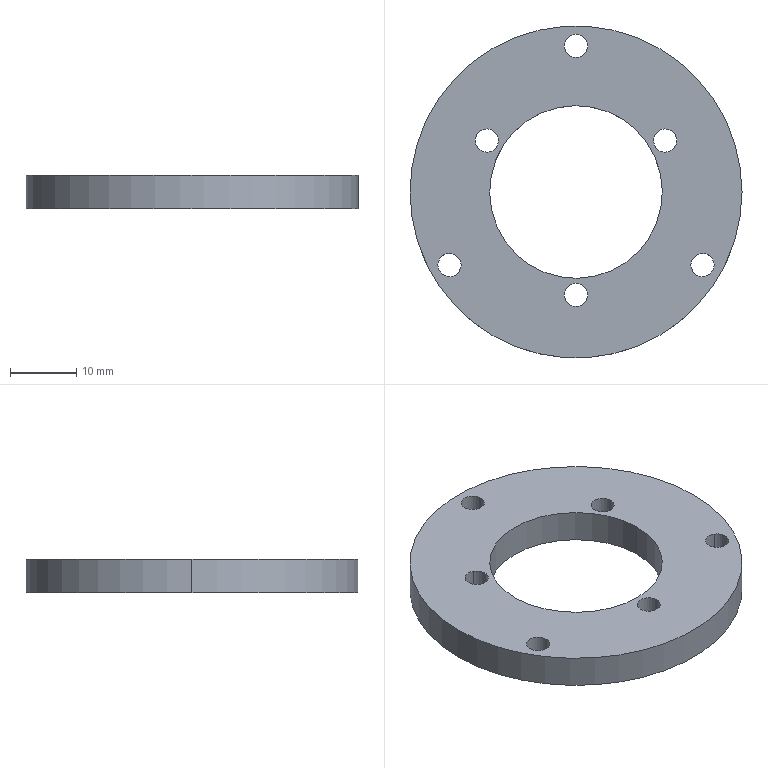Part | SolidWorks | features BaseBody 1 | 1 solid | 18 faces | box 50 x 50 x 5 mm | volume 6874 mm3 | cylinder 16 | plane 2 | commonest cylinder face diameters 3.5 x12 26 x2 50 x2
STEP:
#1=CARTESIAN_POINT('',(326.285,275.622,146.922));
#2=VERTEX_POINT('',#1);
#3=CARTESIAN_POINT('',(328.035,278.653,146.922));
#4=VERTEX_POINT('',#3);
#5=CARTESIAN_POINT('',(327.16,277.138,146.922));
#6=DIRECTION('',(0.,0.,-1.));
#7=DIRECTION('',(0.5,0.866,0.));
#8=AXIS2_PLACEMENT_3D('',#5,#6,#7);
#9=CIRCLE('',#8,1.75);
#10=EDGE_CURVE('',#2,#4,#9,.T.);
#11=ORIENTED_EDGE('',*,*,#10,.F.);
#12=CARTESIAN_POINT('',(326.285,275.622,141.922));
#13=VERTEX_POINT('',#12);
#14=CARTESIAN_POINT('',(326.285,275.622,146.922));
#15=DIRECTION('',(0.,0.,-1.));
#16=VECTOR('',#15,1000.);
#17=LINE('',#14,#16);
#18=EDGE_CURVE('',#2,#13,#17,.T.);
#19=ORIENTED_EDGE('',*,*,#18,.T.);
#20=CARTESIAN_POINT('',(328.035,278.653,141.922));
#21=VERTEX_POINT('',#20);
#22=CARTESIAN_POINT('',(327.16,277.138,141.922));
#23=DIRECTION('',(0.,0.,1.));
#24=DIRECTION('',(-0.5,-0.866,0.));
#25=AXIS2_PLACEMENT_3D('',#22,#23,#24);
#26=CIRCLE('',#25,1.75);
#27=EDGE_CURVE('',#21,#13,#26,.T.);
#28=ORIENTED_EDGE('',*,*,#27,.F.);
#29=CARTESIAN_POINT('',(328.035,278.653,146.922));
#30=DIRECTION('',(0.,0.,-1.));
#31=VECTOR('',#30,1000.);
#32=LINE('',#29,#31);
#33=EDGE_CURVE('',#4,#21,#32,.T.);
#34=ORIENTED_EDGE('',*,*,#33,.F.);
#35=EDGE_LOOP('',(#11,#19,#28,#34));
#36=FACE_OUTER_BOUND('',#35,.T.);
#37=CARTESIAN_POINT('',(327.16,277.138,146.922));
#38=DIRECTION('',(0.,0.,-1.));
#39=DIRECTION('',(0.5,0.866,0.));
#40=AXIS2_PLACEMENT_3D('',#37,#38,#39);
#41=CYLINDRICAL_SURFACE('',#40,1.75);
#42=ADVANCED_FACE('',(#36),#41,.F.);
#43=CARTESIAN_POINT('',(353.132,278.653,146.922));
#44=VERTEX_POINT('',#43);
#45=CARTESIAN_POINT('',(354.882,275.622,146.922));
#46=VERTEX_POINT('',#45);
#47=CARTESIAN_POINT('',(354.007,277.138,146.922));
#48=DIRECTION('',(0.,0.,-1.));
#49=DIRECTION('',(-0.5,0.866,0.));
#50=AXIS2_PLACEMENT_3D('',#47,#48,#49);
#51=CIRCLE('',#50,1.75);
#52=EDGE_CURVE('',#44,#46,#51,.T.);
#53=ORIENTED_EDGE('',*,*,#52,.F.);
#54=CARTESIAN_POINT('',(353.132,278.653,141.922));
#55=VERTEX_POINT('',#54);
#56=CARTESIAN_POINT('',(353.132,278.653,146.922));
#57=DIRECTION('',(0.,0.,-1.));
#58=VECTOR('',#57,1000.);
#59=LINE('',#56,#58);
#60=EDGE_CURVE('',#44,#55,#59,.T.);
#61=ORIENTED_EDGE('',*,*,#60,.T.);
#62=CARTESIAN_POINT('',(354.882,275.622,141.922));
#63=VERTEX_POINT('',#62);
#64=CARTESIAN_POINT('',(354.007,277.138,141.922));
#65=DIRECTION('',(0.,0.,1.));
#66=DIRECTION('',(-0.5,0.866,0.));
#67=AXIS2_PLACEMENT_3D('',#64,#65,#66);
#68=CIRCLE('',#67,1.75);
#69=EDGE_CURVE('',#63,#55,#68,.T.);
#70=ORIENTED_EDGE('',*,*,#69,.F.);
#71=CARTESIAN_POINT('',(354.882,275.622,146.922));
#72=DIRECTION('',(0.,0.,-1.));
#73=VECTOR('',#72,1000.);
#74=LINE('',#71,#73);
#75=EDGE_CURVE('',#46,#63,#74,.T.);
#76=ORIENTED_EDGE('',*,*,#75,.F.);
#77=EDGE_LOOP('',(#53,#61,#70,#76));
#78=FACE_OUTER_BOUND('',#77,.T.);
#79=CARTESIAN_POINT('',(354.007,277.138,146.922));
#80=DIRECTION('',(0.,0.,-1.));
#81=DIRECTION('',(0.5,-0.866,0.));
#82=AXIS2_PLACEMENT_3D('',#79,#80,#81);
#83=CYLINDRICAL_SURFACE('',#82,1.75);
#84=ADVANCED_FACE('',(#78),#83,.F.);
#85=CARTESIAN_POINT('',(342.333,253.888,146.922));
#86=VERTEX_POINT('',#85);
#87=CARTESIAN_POINT('',(338.833,253.888,146.922));
#88=VERTEX_POINT('',#87);
#89=CARTESIAN_POINT('',(340.583,253.888,146.922));
#90=DIRECTION('',(0.,0.,-1.));
#91=DIRECTION('',(1.,0.,0.));
#92=AXIS2_PLACEMENT_3D('',#89,#90,#91);
#93=CIRCLE('',#92,1.75);
#94=EDGE_CURVE('',#86,#88,#93,.T.);
#95=ORIENTED_EDGE('',*,*,#94,.F.);
#96=CARTESIAN_POINT('',(342.333,253.888,141.922));
#97=VERTEX_POINT('',#96);
#98=CARTESIAN_POINT('',(342.333,253.888,146.922));
#99=DIRECTION('',(0.,0.,-1.));
#100=VECTOR('',#99,1000.);
#101=LINE('',#98,#100);
#102=EDGE_CURVE('',#86,#97,#101,.T.);
#103=ORIENTED_EDGE('',*,*,#102,.T.);
#104=CARTESIAN_POINT('',(338.833,253.888,141.922));
#105=VERTEX_POINT('',#104);
#106=CARTESIAN_POINT('',(340.583,253.888,141.922));
#107=DIRECTION('',(0.,0.,1.));
#108=DIRECTION('',(1.,0.,0.));
#109=AXIS2_PLACEMENT_3D('',#106,#107,#108);
#110=CIRCLE('',#109,1.75);
#111=EDGE_CURVE('',#105,#97,#110,.T.);
#112=ORIENTED_EDGE('',*,*,#111,.F.);
#113=CARTESIAN_POINT('',(338.833,253.888,146.922));
#114=DIRECTION('',(0.,0.,-1.));
#115=VECTOR('',#114,1000.);
#116=LINE('',#113,#115);
#117=EDGE_CURVE('',#88,#105,#116,.T.);
#118=ORIENTED_EDGE('',*,*,#117,.F.);
#119=EDGE_LOOP('',(#95,#103,#112,#118));
#120=FACE_OUTER_BOUND('',#119,.T.);
#121=CARTESIAN_POINT('',(340.583,253.888,146.922));
#122=DIRECTION('',(0.,0.,-1.));
#123=DIRECTION('',(-1.,0.,0.));
#124=AXIS2_PLACEMENT_3D('',#121,#122,#123);
#125=CYLINDRICAL_SURFACE('',#124,1.75);
#126=ADVANCED_FACE('',(#120),#125,.F.);
#127=CARTESIAN_POINT('',(358.761,256.872,146.922));
#128=VERTEX_POINT('',#127);
#129=CARTESIAN_POINT('',(360.511,259.903,146.922));
#130=VERTEX_POINT('',#129);
#131=CARTESIAN_POINT('',(359.636,258.388,146.922));
#132=DIRECTION('',(0.,0.,-1.));
#133=DIRECTION('',(-0.5,-0.866,0.));
#134=AXIS2_PLACEMENT_3D('',#131,#132,#133);
#135=CIRCLE('',#134,1.75);
#136=EDGE_CURVE('',#128,#130,#135,.T.);
#137=ORIENTED_EDGE('',*,*,#136,.F.);
#138=CARTESIAN_POINT('',(358.761,256.872,141.922));
#139=VERTEX_POINT('',#138);
#140=CARTESIAN_POINT('',(358.761,256.872,146.922));
#141=DIRECTION('',(0.,0.,-1.));
#142=VECTOR('',#141,1000.);
#143=LINE('',#140,#142);
#144=EDGE_CURVE('',#128,#139,#143,.T.);
#145=ORIENTED_EDGE('',*,*,#144,.T.);
#146=CARTESIAN_POINT('',(360.511,259.903,141.922));
#147=VERTEX_POINT('',#146);
#148=CARTESIAN_POINT('',(359.636,258.388,141.922));
#149=DIRECTION('',(0.,0.,1.));
#150=DIRECTION('',(-0.5,-0.866,0.));
#151=AXIS2_PLACEMENT_3D('',#148,#149,#150);
#152=CIRCLE('',#151,1.75);
#153=EDGE_CURVE('',#147,#139,#152,.T.);
#154=ORIENTED_EDGE('',*,*,#153,.F.);
#155=CARTESIAN_POINT('',(360.511,259.903,146.922));
#156=DIRECTION('',(0.,0.,-1.));
#157=VECTOR('',#156,1000.);
#158=LINE('',#155,#157);
#159=EDGE_CURVE('',#130,#147,#158,.T.);
#160=ORIENTED_EDGE('',*,*,#159,.F.);
#161=EDGE_LOOP('',(#137,#145,#154,#160));
#162=FACE_OUTER_BOUND('',#161,.T.);
#163=CARTESIAN_POINT('',(359.636,258.388,146.922));
#164=DIRECTION('',(0.,0.,-1.));
#165=DIRECTION('',(0.5,0.866,0.));
#166=AXIS2_PLACEMENT_3D('',#163,#164,#165);
#167=CYLINDRICAL_SURFACE('',#166,1.75);
#168=ADVANCED_FACE('',(#162),#167,.F.);
#169=CARTESIAN_POINT('',(320.656,259.903,146.922));
#170=VERTEX_POINT('',#169);
#171=CARTESIAN_POINT('',(322.406,256.872,146.922));
#172=VERTEX_POINT('',#171);
#173=CARTESIAN_POINT('',(321.531,258.388,146.922));
#174=DIRECTION('',(0.,0.,-1.));
#175=DIRECTION('',(-0.5,0.866,0.));
#176=AXIS2_PLACEMENT_3D('',#173,#174,#175);
#177=CIRCLE('',#176,1.75);
#178=EDGE_CURVE('',#170,#172,#177,.T.);
#179=ORIENTED_EDGE('',*,*,#178,.F.);
#180=CARTESIAN_POINT('',(320.656,259.903,141.922));
#181=VERTEX_POINT('',#180);
#182=CARTESIAN_POINT('',(320.656,259.903,146.922));
#183=DIRECTION('',(0.,0.,-1.));
#184=VECTOR('',#183,1000.);
#185=LINE('',#182,#184);
#186=EDGE_CURVE('',#170,#181,#185,.T.);
#187=ORIENTED_EDGE('',*,*,#186,.T.);
#188=CARTESIAN_POINT('',(322.406,256.872,141.922));
#189=VERTEX_POINT('',#188);
#190=CARTESIAN_POINT('',(321.531,258.388,141.922));
#191=DIRECTION('',(0.,0.,1.));
#192=DIRECTION('',(-0.5,0.866,0.));
#193=AXIS2_PLACEMENT_3D('',#190,#191,#192);
#194=CIRCLE('',#193,1.75);
#195=EDGE_CURVE('',#189,#181,#194,.T.);
#196=ORIENTED_EDGE('',*,*,#195,.F.);
#197=CARTESIAN_POINT('',(322.406,256.872,146.922));
#198=DIRECTION('',(0.,0.,-1.));
#199=VECTOR('',#198,1000.);
#200=LINE('',#197,#199);
#201=EDGE_CURVE('',#172,#189,#200,.T.);
#202=ORIENTED_EDGE('',*,*,#201,.F.);
#203=EDGE_LOOP('',(#179,#187,#196,#202));
#204=FACE_OUTER_BOUND('',#203,.T.);
#205=CARTESIAN_POINT('',(321.531,258.388,146.922));
#206=DIRECTION('',(0.,0.,-1.));
#207=DIRECTION('',(0.5,-0.866,0.));
#208=AXIS2_PLACEMENT_3D('',#205,#206,#207);
#209=CYLINDRICAL_SURFACE('',#208,1.75);
#210=ADVANCED_FACE('',(#204),#209,.F.);
#211=CARTESIAN_POINT('',(342.333,291.388,146.922));
#212=VERTEX_POINT('',#211);
#213=CARTESIAN_POINT('',(338.833,291.388,146.922));
#214=VERTEX_POINT('',#213);
#215=CARTESIAN_POINT('',(340.583,291.388,146.922));
#216=DIRECTION('',(0.,0.,-1.));
#217=DIRECTION('',(1.,0.,0.));
#218=AXIS2_PLACEMENT_3D('',#215,#216,#217);
#219=CIRCLE('',#218,1.75);
#220=EDGE_CURVE('',#212,#214,#219,.T.);
#221=ORIENTED_EDGE('',*,*,#220,.F.);
#222=CARTESIAN_POINT('',(342.333,291.388,141.922));
#223=VERTEX_POINT('',#222);
#224=CARTESIAN_POINT('',(342.333,291.388,146.922));
#225=DIRECTION('',(0.,0.,-1.));
#226=VECTOR('',#225,1000.);
#227=LINE('',#224,#226);
#228=EDGE_CURVE('',#212,#223,#227,.T.);
#229=ORIENTED_EDGE('',*,*,#228,.T.);
#230=CARTESIAN_POINT('',(338.833,291.388,141.922));
#231=VERTEX_POINT('',#230);
#232=CARTESIAN_POINT('',(340.583,291.388,141.922));
#233=DIRECTION('',(0.,0.,1.));
#234=DIRECTION('',(1.,0.,0.));
#235=AXIS2_PLACEMENT_3D('',#232,#233,#234);
#236=CIRCLE('',#235,1.75);
#237=EDGE_CURVE('',#231,#223,#236,.T.);
#238=ORIENTED_EDGE('',*,*,#237,.F.);
#239=CARTESIAN_POINT('',(338.833,291.388,146.922));
#240=DIRECTION('',(0.,0.,-1.));
#241=VECTOR('',#240,1000.);
#242=LINE('',#239,#241);
#243=EDGE_CURVE('',#214,#231,#242,.T.);
#244=ORIENTED_EDGE('',*,*,#243,.F.);
#245=EDGE_LOOP('',(#221,#229,#238,#244));
#246=FACE_OUTER_BOUND('',#245,.T.);
#247=CARTESIAN_POINT('',(340.583,291.388,146.922));
#248=DIRECTION('',(0.,0.,-1.));
#249=DIRECTION('',(-1.,0.,0.));
#250=AXIS2_PLACEMENT_3D('',#247,#248,#249);
#251=CYLINDRICAL_SURFACE('',#250,1.75);
#252=ADVANCED_FACE('',(#246),#251,.F.);
#253=CARTESIAN_POINT('',(327.584,269.222,141.922));
#254=VERTEX_POINT('',#253);
#255=CARTESIAN_POINT('',(353.582,269.554,141.922));
#256=VERTEX_POINT('',#255);
#257=CARTESIAN_POINT('',(340.583,269.388,141.922));
#258=DIRECTION('',(0.,0.,1.));
#259=DIRECTION('',(-0.9999,-0.01276,0.));
#260=AXIS2_PLACEMENT_3D('',#257,#258,#259);
#261=CIRCLE('',#260,13.);
#262=EDGE_CURVE('',#254,#256,#261,.T.);
#263=ORIENTED_EDGE('',*,*,#262,.F.);
#264=CARTESIAN_POINT('',(327.584,269.222,146.922));
#265=VERTEX_POINT('',#264);
#266=CARTESIAN_POINT('',(327.584,269.222,68.447));
#267=DIRECTION('',(0.,0.,1.));
#268=VECTOR('',#267,1000.);
#269=LINE('',#266,#268);
#270=EDGE_CURVE('',#254,#265,#269,.T.);
#271=ORIENTED_EDGE('',*,*,#270,.T.);
#272=CARTESIAN_POINT('',(353.582,269.554,146.922));
#273=VERTEX_POINT('',#272);
#274=CARTESIAN_POINT('',(340.583,269.388,146.922));
#275=DIRECTION('',(0.,0.,1.));
#276=DIRECTION('',(-1.,0.,0.));
#277=AXIS2_PLACEMENT_3D('',#274,#275,#276);
#278=CIRCLE('',#277,13.);
#279=EDGE_CURVE('',#265,#273,#278,.T.);
#280=ORIENTED_EDGE('',*,*,#279,.T.);
#281=CARTESIAN_POINT('',(353.582,269.554,68.447));
#282=DIRECTION('',(0.,0.,1.));
#283=VECTOR('',#282,1000.);
#284=LINE('',#281,#283);
#285=EDGE_CURVE('',#256,#273,#284,.T.);
#286=ORIENTED_EDGE('',*,*,#285,.F.);
#287=EDGE_LOOP('',(#263,#271,#280,#286));
#288=FACE_OUTER_BOUND('',#287,.T.);
#289=CARTESIAN_POINT('',(340.583,269.388,68.447));
#290=DIRECTION('',(0.,0.,1.));
#291=DIRECTION('',(0.9999,0.01276,0.));
#292=AXIS2_PLACEMENT_3D('',#289,#290,#291);
#293=CYLINDRICAL_SURFACE('',#292,13.);
#294=ADVANCED_FACE('',(#288),#293,.F.);
#295=CARTESIAN_POINT('',(315.583,269.388,141.922));
#296=VERTEX_POINT('',#295);
#297=CARTESIAN_POINT('',(365.583,269.388,141.922));
#298=VERTEX_POINT('',#297);
#299=CARTESIAN_POINT('',(340.583,269.388,141.922));
#300=DIRECTION('',(0.,0.,-1.));
#301=DIRECTION('',(1.,0.,0.));
#302=AXIS2_PLACEMENT_3D('',#299,#300,#301);
#303=CIRCLE('',#302,25.);
#304=EDGE_CURVE('',#296,#298,#303,.T.);
#305=ORIENTED_EDGE('',*,*,#304,.F.);
#306=CARTESIAN_POINT('',(315.583,269.388,146.922));
#307=VERTEX_POINT('',#306);
#308=CARTESIAN_POINT('',(315.583,269.388,141.922));
#309=DIRECTION('',(0.,0.,1.));
#310=VECTOR('',#309,1000.);
#311=LINE('',#308,#310);
#312=EDGE_CURVE('',#296,#307,#311,.T.);
#313=ORIENTED_EDGE('',*,*,#312,.T.);
#314=CARTESIAN_POINT('',(365.583,269.388,146.922));
#315=VERTEX_POINT('',#314);
#316=CARTESIAN_POINT('',(340.583,269.388,146.922));
#317=DIRECTION('',(0.,0.,1.));
#318=DIRECTION('',(-1.,0.,0.));
#319=AXIS2_PLACEMENT_3D('',#316,#317,#318);
#320=CIRCLE('',#319,25.);
#321=EDGE_CURVE('',#315,#307,#320,.T.);
#322=ORIENTED_EDGE('',*,*,#321,.F.);
#323=CARTESIAN_POINT('',(365.583,269.388,141.922));
#324=DIRECTION('',(0.,0.,1.));
#325=VECTOR('',#324,1000.);
#326=LINE('',#323,#325);
#327=EDGE_CURVE('',#298,#315,#326,.T.);
#328=ORIENTED_EDGE('',*,*,#327,.F.);
#329=EDGE_LOOP('',(#305,#313,#322,#328));
#330=FACE_OUTER_BOUND('',#329,.T.);
#331=CARTESIAN_POINT('',(340.583,269.388,141.922));
#332=DIRECTION('',(0.,0.,1.));
#333=DIRECTION('',(1.,0.,0.));
#334=AXIS2_PLACEMENT_3D('',#331,#332,#333);
#335=CYLINDRICAL_SURFACE('',#334,25.);
#336=ADVANCED_FACE('',(#330),#335,.T.);
#337=ORIENTED_EDGE('',*,*,#312,.F.);
#338=CARTESIAN_POINT('',(340.583,269.388,141.922));
#339=DIRECTION('',(0.,0.,-1.));
#340=DIRECTION('',(1.,0.,0.));
#341=AXIS2_PLACEMENT_3D('',#338,#339,#340);
#342=CIRCLE('',#341,25.);
#343=EDGE_CURVE('',#298,#296,#342,.T.);
#344=ORIENTED_EDGE('',*,*,#343,.F.);
#345=ORIENTED_EDGE('',*,*,#327,.T.);
#346=CARTESIAN_POINT('',(340.583,269.388,146.922));
#347=DIRECTION('',(0.,0.,1.));
#348=DIRECTION('',(-1.,0.,0.));
#349=AXIS2_PLACEMENT_3D('',#346,#347,#348);
#350=CIRCLE('',#349,25.);
#351=EDGE_CURVE('',#307,#315,#350,.T.);
#352=ORIENTED_EDGE('',*,*,#351,.F.);
#353=EDGE_LOOP('',(#337,#344,#345,#352));
#354=FACE_OUTER_BOUND('',#353,.T.);
#355=CARTESIAN_POINT('',(340.583,269.388,141.922));
#356=DIRECTION('',(0.,0.,1.));
#357=DIRECTION('',(1.,0.,0.));
#358=AXIS2_PLACEMENT_3D('',#355,#356,#357);
#359=CYLINDRICAL_SURFACE('',#358,25.);
#360=ADVANCED_FACE('',(#354),#359,.T.);
#361=ORIENTED_EDGE('',*,*,#270,.F.);
#362=CARTESIAN_POINT('',(340.583,269.388,141.922));
#363=DIRECTION('',(0.,0.,1.));
#364=DIRECTION('',(-0.9999,-0.01276,0.));
#365=AXIS2_PLACEMENT_3D('',#362,#363,#364);
#366=CIRCLE('',#365,13.);
#367=EDGE_CURVE('',#256,#254,#366,.T.);
#368=ORIENTED_EDGE('',*,*,#367,.F.);
#369=ORIENTED_EDGE('',*,*,#285,.T.);
#370=CARTESIAN_POINT('',(340.583,269.388,146.922));
#371=DIRECTION('',(0.,0.,1.));
#372=DIRECTION('',(-1.,0.,0.));
#373=AXIS2_PLACEMENT_3D('',#370,#371,#372);
#374=CIRCLE('',#373,13.);
#375=EDGE_CURVE('',#273,#265,#374,.T.);
#376=ORIENTED_EDGE('',*,*,#375,.T.);
#377=EDGE_LOOP('',(#361,#368,#369,#376));
#378=FACE_OUTER_BOUND('',#377,.T.);
#379=CARTESIAN_POINT('',(340.583,269.388,68.447));
#380=DIRECTION('',(0.,0.,1.));
#381=DIRECTION('',(0.9999,0.01276,0.));
#382=AXIS2_PLACEMENT_3D('',#379,#380,#381);
#383=CYLINDRICAL_SURFACE('',#382,13.);
#384=ADVANCED_FACE('',(#378),#383,.F.);
#385=ORIENTED_EDGE('',*,*,#228,.F.);
#386=CARTESIAN_POINT('',(340.583,291.388,146.922));
#387=DIRECTION('',(0.,0.,-1.));
#388=DIRECTION('',(1.,0.,0.));
#389=AXIS2_PLACEMENT_3D('',#386,#387,#388);
#390=CIRCLE('',#389,1.75);
#391=EDGE_CURVE('',#214,#212,#390,.T.);
#392=ORIENTED_EDGE('',*,*,#391,.F.);
#393=ORIENTED_EDGE('',*,*,#243,.T.);
#394=CARTESIAN_POINT('',(340.583,291.388,141.922));
#395=DIRECTION('',(0.,0.,1.));
#396=DIRECTION('',(1.,0.,0.));
#397=AXIS2_PLACEMENT_3D('',#394,#395,#396);
#398=CIRCLE('',#397,1.75);
#399=EDGE_CURVE('',#223,#231,#398,.T.);
#400=ORIENTED_EDGE('',*,*,#399,.F.);
#401=EDGE_LOOP('',(#385,#392,#393,#400));
#402=FACE_OUTER_BOUND('',#401,.T.);
#403=CARTESIAN_POINT('',(340.583,291.388,146.922));
#404=DIRECTION('',(0.,0.,-1.));
#405=DIRECTION('',(-1.,0.,0.));
#406=AXIS2_PLACEMENT_3D('',#403,#404,#405);
#407=CYLINDRICAL_SURFACE('',#406,1.75);
#408=ADVANCED_FACE('',(#402),#407,.F.);
#409=ORIENTED_EDGE('',*,*,#186,.F.);
#410=CARTESIAN_POINT('',(321.531,258.388,146.922));
#411=DIRECTION('',(0.,0.,-1.));
#412=DIRECTION('',(-0.5,0.866,0.));
#413=AXIS2_PLACEMENT_3D('',#410,#411,#412);
#414=CIRCLE('',#413,1.75);
#415=EDGE_CURVE('',#172,#170,#414,.T.);
#416=ORIENTED_EDGE('',*,*,#415,.F.);
#417=ORIENTED_EDGE('',*,*,#201,.T.);
#418=CARTESIAN_POINT('',(321.531,258.388,141.922));
#419=DIRECTION('',(0.,0.,1.));
#420=DIRECTION('',(-0.5,0.866,0.));
#421=AXIS2_PLACEMENT_3D('',#418,#419,#420);
#422=CIRCLE('',#421,1.75);
#423=EDGE_CURVE('',#181,#189,#422,.T.);
#424=ORIENTED_EDGE('',*,*,#423,.F.);
#425=EDGE_LOOP('',(#409,#416,#417,#424));
#426=FACE_OUTER_BOUND('',#425,.T.);
#427=CARTESIAN_POINT('',(321.531,258.388,146.922));
#428=DIRECTION('',(0.,0.,-1.));
#429=DIRECTION('',(0.5,-0.866,0.));
#430=AXIS2_PLACEMENT_3D('',#427,#428,#429);
#431=CYLINDRICAL_SURFACE('',#430,1.75);
#432=ADVANCED_FACE('',(#426),#431,.F.);
#433=ORIENTED_EDGE('',*,*,#144,.F.);
#434=CARTESIAN_POINT('',(359.636,258.388,146.922));
#435=DIRECTION('',(0.,0.,-1.));
#436=DIRECTION('',(-0.5,-0.866,0.));
#437=AXIS2_PLACEMENT_3D('',#434,#435,#436);
#438=CIRCLE('',#437,1.75);
#439=EDGE_CURVE('',#130,#128,#438,.T.);
#440=ORIENTED_EDGE('',*,*,#439,.F.);
#441=ORIENTED_EDGE('',*,*,#159,.T.);
#442=CARTESIAN_POINT('',(359.636,258.388,141.922));
#443=DIRECTION('',(0.,0.,1.));
#444=DIRECTION('',(-0.5,-0.866,0.));
#445=AXIS2_PLACEMENT_3D('',#442,#443,#444);
#446=CIRCLE('',#445,1.75);
#447=EDGE_CURVE('',#139,#147,#446,.T.);
#448=ORIENTED_EDGE('',*,*,#447,.F.);
#449=EDGE_LOOP('',(#433,#440,#441,#448));
#450=FACE_OUTER_BOUND('',#449,.T.);
#451=CARTESIAN_POINT('',(359.636,258.388,146.922));
#452=DIRECTION('',(0.,0.,-1.));
#453=DIRECTION('',(0.5,0.866,0.));
#454=AXIS2_PLACEMENT_3D('',#451,#452,#453);
#455=CYLINDRICAL_SURFACE('',#454,1.75);
#456=ADVANCED_FACE('',(#450),#455,.F.);
#457=ORIENTED_EDGE('',*,*,#102,.F.);
#458=CARTESIAN_POINT('',(340.583,253.888,146.922));
#459=DIRECTION('',(0.,0.,-1.));
#460=DIRECTION('',(1.,0.,0.));
#461=AXIS2_PLACEMENT_3D('',#458,#459,#460);
#462=CIRCLE('',#461,1.75);
#463=EDGE_CURVE('',#88,#86,#462,.T.);
#464=ORIENTED_EDGE('',*,*,#463,.F.);
#465=ORIENTED_EDGE('',*,*,#117,.T.);
#466=CARTESIAN_POINT('',(340.583,253.888,141.922));
#467=DIRECTION('',(0.,0.,1.));
#468=DIRECTION('',(1.,0.,0.));
#469=AXIS2_PLACEMENT_3D('',#466,#467,#468);
#470=CIRCLE('',#469,1.75);
#471=EDGE_CURVE('',#97,#105,#470,.T.);
#472=ORIENTED_EDGE('',*,*,#471,.F.);
#473=EDGE_LOOP('',(#457,#464,#465,#472));
#474=FACE_OUTER_BOUND('',#473,.T.);
#475=CARTESIAN_POINT('',(340.583,253.888,146.922));
#476=DIRECTION('',(0.,0.,-1.));
#477=DIRECTION('',(-1.,0.,0.));
#478=AXIS2_PLACEMENT_3D('',#475,#476,#477);
#479=CYLINDRICAL_SURFACE('',#478,1.75);
#480=ADVANCED_FACE('',(#474),#479,.F.);
#481=ORIENTED_EDGE('',*,*,#60,.F.);
#482=CARTESIAN_POINT('',(354.007,277.138,146.922));
#483=DIRECTION('',(0.,0.,-1.));
#484=DIRECTION('',(-0.5,0.866,0.));
#485=AXIS2_PLACEMENT_3D('',#482,#483,#484);
#486=CIRCLE('',#485,1.75);
#487=EDGE_CURVE('',#46,#44,#486,.T.);
#488=ORIENTED_EDGE('',*,*,#487,.F.);
#489=ORIENTED_EDGE('',*,*,#75,.T.);
#490=CARTESIAN_POINT('',(354.007,277.138,141.922));
#491=DIRECTION('',(0.,0.,1.));
#492=DIRECTION('',(-0.5,0.866,0.));
#493=AXIS2_PLACEMENT_3D('',#490,#491,#492);
#494=CIRCLE('',#493,1.75);
#495=EDGE_CURVE('',#55,#63,#494,.T.);
#496=ORIENTED_EDGE('',*,*,#495,.F.);
#497=EDGE_LOOP('',(#481,#488,#489,#496));
#498=FACE_OUTER_BOUND('',#497,.T.);
#499=CARTESIAN_POINT('',(354.007,277.138,146.922));
#500=DIRECTION('',(0.,0.,-1.));
#501=DIRECTION('',(0.5,-0.866,0.));
#502=AXIS2_PLACEMENT_3D('',#499,#500,#501);
#503=CYLINDRICAL_SURFACE('',#502,1.75);
#504=ADVANCED_FACE('',(#498),#503,.F.);
#505=CARTESIAN_POINT('',(327.16,277.138,146.922));
#506=DIRECTION('',(0.,0.,-1.));
#507=DIRECTION('',(0.5,0.866,0.));
#508=AXIS2_PLACEMENT_3D('',#505,#506,#507);
#509=CIRCLE('',#508,1.75);
#510=EDGE_CURVE('',#4,#2,#509,.T.);
#511=ORIENTED_EDGE('',*,*,#510,.T.);
#512=ORIENTED_EDGE('',*,*,#10,.T.);
#513=EDGE_LOOP('',(#511,#512));
#514=FACE_BOUND('',#513,.T.);
#515=ORIENTED_EDGE('',*,*,#375,.F.);
#516=ORIENTED_EDGE('',*,*,#279,.F.);
#517=EDGE_LOOP('',(#515,#516));
#518=FACE_BOUND('',#517,.T.);
#519=ORIENTED_EDGE('',*,*,#391,.T.);
#520=ORIENTED_EDGE('',*,*,#220,.T.);
#521=EDGE_LOOP('',(#519,#520));
#522=FACE_BOUND('',#521,.T.);
#523=ORIENTED_EDGE('',*,*,#415,.T.);
#524=ORIENTED_EDGE('',*,*,#178,.T.);
#525=EDGE_LOOP('',(#523,#524));
#526=FACE_BOUND('',#525,.T.);
#527=ORIENTED_EDGE('',*,*,#439,.T.);
#528=ORIENTED_EDGE('',*,*,#136,.T.);
#529=EDGE_LOOP('',(#527,#528));
#530=FACE_BOUND('',#529,.T.);
#531=ORIENTED_EDGE('',*,*,#463,.T.);
#532=ORIENTED_EDGE('',*,*,#94,.T.);
#533=EDGE_LOOP('',(#531,#532));
#534=FACE_BOUND('',#533,.T.);
#535=ORIENTED_EDGE('',*,*,#487,.T.);
#536=ORIENTED_EDGE('',*,*,#52,.T.);
#537=EDGE_LOOP('',(#535,#536));
#538=FACE_BOUND('',#537,.T.);
#539=ORIENTED_EDGE('',*,*,#321,.T.);
#540=ORIENTED_EDGE('',*,*,#351,.T.);
#541=EDGE_LOOP('',(#539,#540));
#542=FACE_OUTER_BOUND('',#541,.T.);
#543=CARTESIAN_POINT('',(340.583,269.388,146.922));
#544=DIRECTION('',(0.,0.,1.));
#545=DIRECTION('',(1.,0.,0.));
#546=AXIS2_PLACEMENT_3D('',#543,#544,#545);
#547=PLANE('',#546);
#548=ADVANCED_FACE('',(#514,#518,#522,#526,#530,#534,#538,#542),#547,.T.);
#549=ORIENTED_EDGE('',*,*,#27,.T.);
#550=CARTESIAN_POINT('',(327.16,277.138,141.922));
#551=DIRECTION('',(0.,0.,1.));
#552=DIRECTION('',(-0.5,-0.866,0.));
#553=AXIS2_PLACEMENT_3D('',#550,#551,#552);
#554=CIRCLE('',#553,1.75);
#555=EDGE_CURVE('',#13,#21,#554,.T.);
#556=ORIENTED_EDGE('',*,*,#555,.T.);
#557=EDGE_LOOP('',(#549,#556));
#558=FACE_BOUND('',#557,.T.);
#559=ORIENTED_EDGE('',*,*,#367,.T.);
#560=ORIENTED_EDGE('',*,*,#262,.T.);
#561=EDGE_LOOP('',(#559,#560));
#562=FACE_BOUND('',#561,.T.);
#563=ORIENTED_EDGE('',*,*,#237,.T.);
#564=ORIENTED_EDGE('',*,*,#399,.T.);
#565=EDGE_LOOP('',(#563,#564));
#566=FACE_BOUND('',#565,.T.);
#567=ORIENTED_EDGE('',*,*,#195,.T.);
#568=ORIENTED_EDGE('',*,*,#423,.T.);
#569=EDGE_LOOP('',(#567,#568));
#570=FACE_BOUND('',#569,.T.);
#571=ORIENTED_EDGE('',*,*,#153,.T.);
#572=ORIENTED_EDGE('',*,*,#447,.T.);
#573=EDGE_LOOP('',(#571,#572));
#574=FACE_BOUND('',#573,.T.);
#575=ORIENTED_EDGE('',*,*,#111,.T.);
#576=ORIENTED_EDGE('',*,*,#471,.T.);
#577=EDGE_LOOP('',(#575,#576));
#578=FACE_BOUND('',#577,.T.);
#579=ORIENTED_EDGE('',*,*,#69,.T.);
#580=ORIENTED_EDGE('',*,*,#495,.T.);
#581=EDGE_LOOP('',(#579,#580));
#582=FACE_BOUND('',#581,.T.);
#583=ORIENTED_EDGE('',*,*,#343,.T.);
#584=ORIENTED_EDGE('',*,*,#304,.T.);
#585=EDGE_LOOP('',(#583,#584));
#586=FACE_OUTER_BOUND('',#585,.T.);
#587=CARTESIAN_POINT('',(340.583,269.388,141.922));
#588=DIRECTION('',(0.,0.,-1.));
#589=DIRECTION('',(0.,-1.,0.));
#590=AXIS2_PLACEMENT_3D('',#587,#588,#589);
#591=PLANE('',#590);
#592=ADVANCED_FACE('',(#558,#562,#566,#570,#574,#578,#582,#586),#591,.T.);
#593=ORIENTED_EDGE('',*,*,#18,.F.);
#594=ORIENTED_EDGE('',*,*,#510,.F.);
#595=ORIENTED_EDGE('',*,*,#33,.T.);
#596=ORIENTED_EDGE('',*,*,#555,.F.);
#597=EDGE_LOOP('',(#593,#594,#595,#596));
#598=FACE_OUTER_BOUND('',#597,.T.);
#599=CARTESIAN_POINT('',(327.16,277.138,146.922));
#600=DIRECTION('',(0.,0.,-1.));
#601=DIRECTION('',(0.5,0.866,0.));
#602=AXIS2_PLACEMENT_3D('',#599,#600,#601);
#603=CYLINDRICAL_SURFACE('',#602,1.75);
#604=ADVANCED_FACE('',(#598),#603,.F.);
#605=CLOSED_SHELL('',(#42,#84,#126,#168,#210,#252,#294,#336,#360,#384,#408,#432,#456,#480,#504,#548,#592,#604));
#606=MANIFOLD_SOLID_BREP('',#605);
#607=CARTESIAN_POINT('',(0.,0.,0.));
#608=DIRECTION('',(0.,0.,1.));
#609=DIRECTION('',(1.,0.,0.));
#610=AXIS2_PLACEMENT_3D('',#607,#608,#609);
#611=(LENGTH_UNIT()NAMED_UNIT(*)SI_UNIT(.MILLI.,.METRE.));
#612=UNCERTAINTY_MEASURE_WITH_UNIT(LENGTH_MEASURE(0.00001),#611,'','');
#613=(NAMED_UNIT(*)PLANE_ANGLE_UNIT()SI_UNIT($,.RADIAN.));
#614=(NAMED_UNIT(*)SI_UNIT($,.STERADIAN.)SOLID_ANGLE_UNIT());
#615=(GEOMETRIC_REPRESENTATION_CONTEXT(3)GLOBAL_UNCERTAINTY_ASSIGNED_CONTEXT((#612))GLOBAL_UNIT_ASSIGNED_CONTEXT((#611,#613,#614))REPRESENTATION_CONTEXT('',''));
#616=ADVANCED_BREP_SHAPE_REPRESENTATION('',(#606,#610),#615);